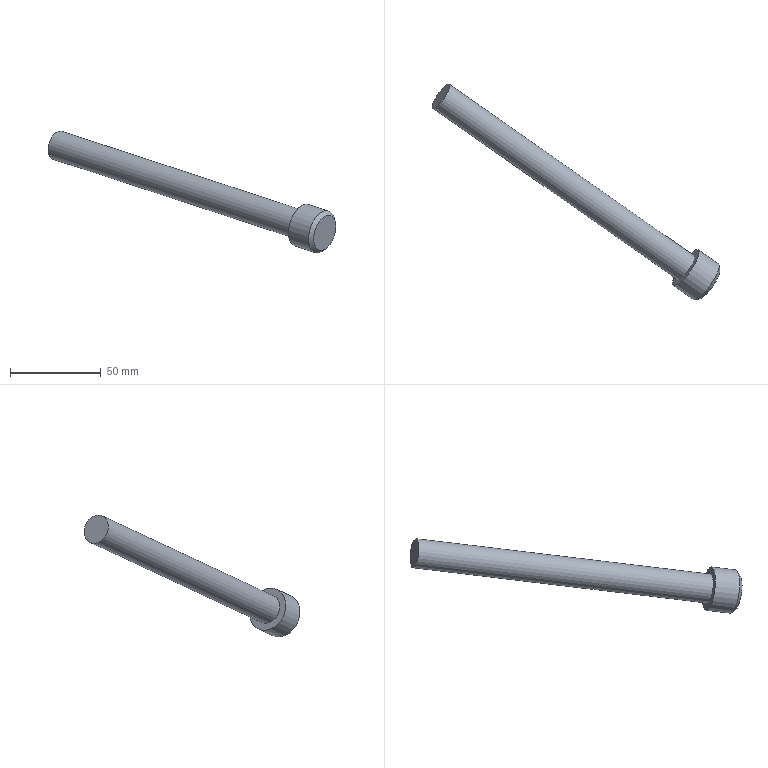Part | NX | features solid 2 | 1 solid | 6 faces | box 158.178 x 118.592 x 66.941 mm | volume 41276 mm3 | plane 3 | cylinder 2 | cone 1 | commonest cylinder face diameters 16 x1 24 x1
STEP:
#1=CARTESIAN_POINT('',(-664.717,367.778,-149.571));
#2=VERTEX_POINT('',#1);
#3=CARTESIAN_POINT('',(-670.453,359.586,-149.571));
#4=DIRECTION('',(0.7912,-0.554,-0.2588));
#5=DIRECTION('',(0.5736,0.8192,0.));
#6=AXIS2_PLACEMENT_3D('',#3,#4,#5);
#7=CIRCLE('',#6,10.);
#8=EDGE_CURVE('',#2,#2,#7,.T.);
#9=ORIENTED_EDGE('',*,*,#8,.T.);
#10=EDGE_LOOP('',(#9));
#11=FACE_BOUND('',#10,.T.);
#12=CARTESIAN_POINT('',(-670.453,359.586,-149.571));
#13=DIRECTION('',(0.7912,-0.554,-0.2588));
#14=DIRECTION('',(0.5736,0.8192,0.));
#15=AXIS2_PLACEMENT_3D('',#12,#13,#14);
#16=PLANE('',#15);
#17=ADVANCED_FACE('',(#11),#16,.T.);
#18=CARTESIAN_POINT('',(-687.701,361.898,-145.43));
#19=VERTEX_POINT('',#18);
#20=CARTESIAN_POINT('',(-683.113,368.451,-145.43));
#21=DIRECTION('',(-0.7912,0.554,0.2588));
#22=DIRECTION('',(-0.5736,-0.8192,0.));
#23=AXIS2_PLACEMENT_3D('',#20,#21,#22);
#24=CIRCLE('',#23,8.);
#25=EDGE_CURVE('',#19,#19,#24,.T.);
#26=ORIENTED_EDGE('',*,*,#25,.F.);
#27=EDGE_LOOP('',(#26));
#28=FACE_BOUND('',#27,.T.);
#29=CARTESIAN_POINT('',(-676.23,378.281,-145.43));
#30=VERTEX_POINT('',#29);
#31=CARTESIAN_POINT('',(-683.113,368.451,-145.43));
#32=DIRECTION('',(0.7912,-0.554,-0.2588));
#33=DIRECTION('',(0.5736,0.8192,0.));
#34=AXIS2_PLACEMENT_3D('',#31,#32,#33);
#35=CIRCLE('',#34,12.);
#36=EDGE_CURVE('',#30,#30,#35,.T.);
#37=ORIENTED_EDGE('',*,*,#36,.F.);
#38=EDGE_LOOP('',(#37));
#39=FACE_BOUND('',#38,.T.);
#40=CARTESIAN_POINT('',(-683.113,368.451,-145.43));
#41=DIRECTION('',(-0.7912,0.554,0.2588));
#42=DIRECTION('',(-0.5736,-0.8192,0.));
#43=AXIS2_PLACEMENT_3D('',#40,#41,#42);
#44=PLANE('',#43);
#45=ADVANCED_FACE('',(#28,#39),#44,.T.);
#46=CARTESIAN_POINT('',(-665.152,370.524,-149.053));
#47=VERTEX_POINT('',#46);
#48=CARTESIAN_POINT('',(-672.035,360.695,-149.053));
#49=DIRECTION('',(0.7912,-0.554,-0.2588));
#50=DIRECTION('',(0.5736,0.8192,0.));
#51=AXIS2_PLACEMENT_3D('',#48,#49,#50);
#52=CIRCLE('',#51,12.);
#53=EDGE_CURVE('',#47,#47,#52,.F.);
#54=ORIENTED_EDGE('',*,*,#53,.T.);
#55=EDGE_LOOP('',(#54));
#56=FACE_BOUND('',#55,.T.);
#57=ORIENTED_EDGE('',*,*,#36,.T.);
#58=EDGE_LOOP('',(#57));
#59=FACE_BOUND('',#58,.T.);
#60=CARTESIAN_POINT('',(-683.113,368.451,-145.43));
#61=DIRECTION('',(0.7912,-0.554,-0.2588));
#62=DIRECTION('',(0.5736,0.8192,0.));
#63=AXIS2_PLACEMENT_3D('',#60,#61,#62);
#64=CYLINDRICAL_SURFACE('',#63,12.);
#65=ADVANCED_FACE('',(#56,#59),#64,.T.);
#66=CARTESIAN_POINT('',(-822.212,456.083,-101.43));
#67=VERTEX_POINT('',#66);
#68=CARTESIAN_POINT('',(-817.624,462.636,-101.43));
#69=DIRECTION('',(-0.7912,0.554,0.2588));
#70=DIRECTION('',(-0.5736,-0.8192,0.));
#71=AXIS2_PLACEMENT_3D('',#68,#69,#70);
#72=CIRCLE('',#71,8.);
#73=EDGE_CURVE('',#67,#67,#72,.F.);
#74=ORIENTED_EDGE('',*,*,#73,.F.);
#75=EDGE_LOOP('',(#74));
#76=FACE_BOUND('',#75,.T.);
#77=CARTESIAN_POINT('',(-817.624,462.636,-101.43));
#78=DIRECTION('',(-0.7912,0.554,0.2588));
#79=DIRECTION('',(-0.5736,-0.8192,0.));
#80=AXIS2_PLACEMENT_3D('',#77,#78,#79);
#81=PLANE('',#80);
#82=ADVANCED_FACE('',(#76),#81,.T.);
#83=ORIENTED_EDGE('',*,*,#73,.T.);
#84=EDGE_LOOP('',(#83));
#85=FACE_BOUND('',#84,.T.);
#86=ORIENTED_EDGE('',*,*,#25,.T.);
#87=EDGE_LOOP('',(#86));
#88=FACE_BOUND('',#87,.T.);
#89=CARTESIAN_POINT('',(-683.113,368.451,-145.43));
#90=DIRECTION('',(-0.7912,0.554,0.2588));
#91=DIRECTION('',(-0.5736,-0.8192,0.));
#92=AXIS2_PLACEMENT_3D('',#89,#90,#91);
#93=CYLINDRICAL_SURFACE('',#92,8.);
#94=ADVANCED_FACE('',(#85,#88),#93,.T.);
#95=ORIENTED_EDGE('',*,*,#8,.F.);
#96=EDGE_LOOP('',(#95));
#97=FACE_BOUND('',#96,.T.);
#98=ORIENTED_EDGE('',*,*,#53,.F.);
#99=EDGE_LOOP('',(#98));
#100=FACE_BOUND('',#99,.T.);
#101=CARTESIAN_POINT('',(-672.035,360.695,-149.053));
#102=DIRECTION('',(-0.7912,0.554,0.2588));
#103=DIRECTION('',(-0.5736,-0.8192,0.));
#104=AXIS2_PLACEMENT_3D('',#101,#102,#103);
#105=CONICAL_SURFACE('',#104,12.,0.7854);
#106=ADVANCED_FACE('',(#97,#100),#105,.T.);
#107=CLOSED_SHELL('',(#17,#45,#65,#82,#94,#106));
#108=MANIFOLD_SOLID_BREP('',#107);
#109=(LENGTH_UNIT()NAMED_UNIT(*)SI_UNIT(.MILLI.,.METRE.));
#110=UNCERTAINTY_MEASURE_WITH_UNIT(LENGTH_MEASURE(0.00001),#109,'','');
#111=(NAMED_UNIT(*)PLANE_ANGLE_UNIT()SI_UNIT($,.RADIAN.));
#112=(NAMED_UNIT(*)SI_UNIT($,.STERADIAN.)SOLID_ANGLE_UNIT());
#113=(GEOMETRIC_REPRESENTATION_CONTEXT(3)GLOBAL_UNCERTAINTY_ASSIGNED_CONTEXT((#110))GLOBAL_UNIT_ASSIGNED_CONTEXT((#109,#111,#112))REPRESENTATION_CONTEXT('',''));
#114=ADVANCED_BREP_SHAPE_REPRESENTATION('',(#108),#113);